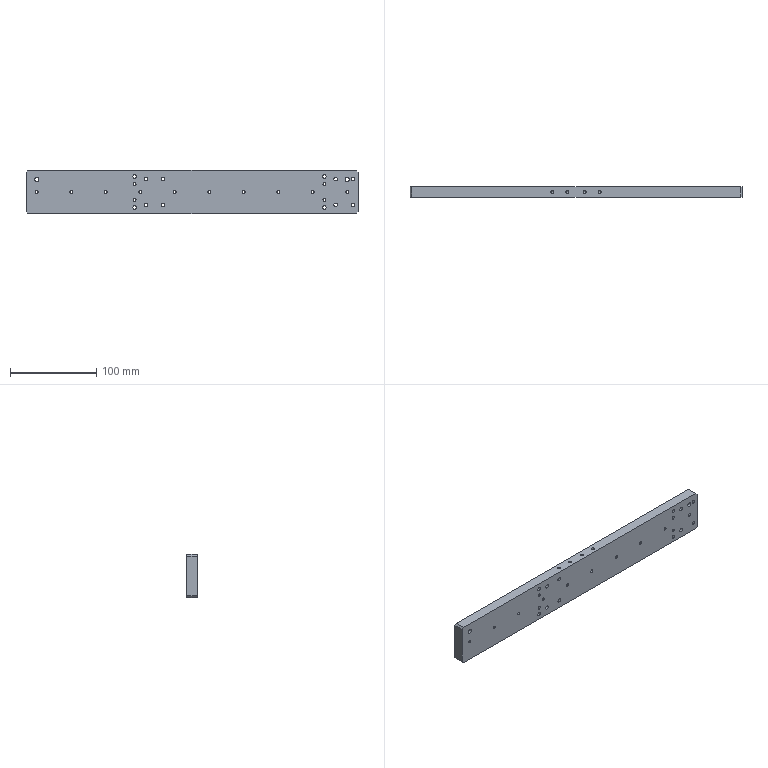Part | 1 solid | 50 faces | box 385 x 12 x 50 mm | volume 226445 mm3 | cylinder 34 | plane 10 | cone 6 | commonest cylinder face diameters 3.3 x20 4.2 x8 4 x4 5 x2
STEP:
#1=CARTESIAN_POINT('',(192.5,-6.,48.));
#2=VERTEX_POINT('',#1);
#3=CARTESIAN_POINT('',(190.5,-6.,50.));
#4=VERTEX_POINT('',#3);
#5=CARTESIAN_POINT('',(190.5,-6.,50.));
#6=DIRECTION('',(-0.7071,0.,0.7071));
#7=VECTOR('',#6,1000.);
#8=LINE('',#5,#7);
#9=EDGE_CURVE('',#2,#4,#8,.T.);
#10=ORIENTED_EDGE('',*,*,#9,.F.);
#11=CARTESIAN_POINT('',(192.5,6.,48.));
#12=VERTEX_POINT('',#11);
#13=CARTESIAN_POINT('',(192.5,-6.,48.));
#14=DIRECTION('',(0.,-1.,0.));
#15=VECTOR('',#14,1000.);
#16=LINE('',#13,#15);
#17=EDGE_CURVE('',#12,#2,#16,.T.);
#18=ORIENTED_EDGE('',*,*,#17,.F.);
#19=CARTESIAN_POINT('',(190.5,6.,50.));
#20=VERTEX_POINT('',#19);
#21=CARTESIAN_POINT('',(190.5,6.,50.));
#22=DIRECTION('',(0.7071,0.,-0.7071));
#23=VECTOR('',#22,1000.);
#24=LINE('',#21,#23);
#25=EDGE_CURVE('',#20,#12,#24,.T.);
#26=ORIENTED_EDGE('',*,*,#25,.F.);
#27=CARTESIAN_POINT('',(190.5,0.,50.));
#28=DIRECTION('',(0.,1.,0.));
#29=VECTOR('',#28,1000.);
#30=LINE('',#27,#29);
#31=EDGE_CURVE('',#4,#20,#30,.T.);
#32=ORIENTED_EDGE('',*,*,#31,.F.);
#33=EDGE_LOOP('',(#10,#18,#26,#32));
#34=FACE_BOUND('',#33,.T.);
#35=CARTESIAN_POINT('',(190.5,0.,50.));
#36=DIRECTION('',(-0.7071,0.,-0.7071));
#37=DIRECTION('',(0.,1.,0.));
#38=AXIS2_PLACEMENT_3D('',#35,#36,#37);
#39=PLANE('',#38);
#40=ADVANCED_FACE('',(#34),#39,.F.);
#41=CARTESIAN_POINT('',(190.5,-6.,0.));
#42=VERTEX_POINT('',#41);
#43=CARTESIAN_POINT('',(192.5,-6.,2.));
#44=VERTEX_POINT('',#43);
#45=CARTESIAN_POINT('',(192.5,-6.,2.));
#46=DIRECTION('',(0.7071,0.,0.7071));
#47=VECTOR('',#46,1000.);
#48=LINE('',#45,#47);
#49=EDGE_CURVE('',#42,#44,#48,.T.);
#50=ORIENTED_EDGE('',*,*,#49,.F.);
#51=CARTESIAN_POINT('',(190.5,6.,0.));
#52=VERTEX_POINT('',#51);
#53=CARTESIAN_POINT('',(190.5,-6.,0.));
#54=DIRECTION('',(0.,-1.,0.));
#55=VECTOR('',#54,1000.);
#56=LINE('',#53,#55);
#57=EDGE_CURVE('',#52,#42,#56,.T.);
#58=ORIENTED_EDGE('',*,*,#57,.F.);
#59=CARTESIAN_POINT('',(192.5,6.,2.));
#60=VERTEX_POINT('',#59);
#61=CARTESIAN_POINT('',(192.5,6.,2.));
#62=DIRECTION('',(-0.7071,0.,-0.7071));
#63=VECTOR('',#62,1000.);
#64=LINE('',#61,#63);
#65=EDGE_CURVE('',#60,#52,#64,.T.);
#66=ORIENTED_EDGE('',*,*,#65,.F.);
#67=CARTESIAN_POINT('',(192.5,6.,2.));
#68=DIRECTION('',(0.,1.,0.));
#69=VECTOR('',#68,1000.);
#70=LINE('',#67,#69);
#71=EDGE_CURVE('',#44,#60,#70,.T.);
#72=ORIENTED_EDGE('',*,*,#71,.F.);
#73=EDGE_LOOP('',(#50,#58,#66,#72));
#74=FACE_BOUND('',#73,.T.);
#75=CARTESIAN_POINT('',(192.5,-6.,2.));
#76=DIRECTION('',(0.7071,0.,-0.7071));
#77=DIRECTION('',(0.,-1.,0.));
#78=AXIS2_PLACEMENT_3D('',#75,#76,#77);
#79=PLANE('',#78);
#80=ADVANCED_FACE('',(#74),#79,.T.);
#81=CARTESIAN_POINT('',(-192.5,6.,48.));
#82=VERTEX_POINT('',#81);
#83=CARTESIAN_POINT('',(-190.5,6.,50.));
#84=VERTEX_POINT('',#83);
#85=CARTESIAN_POINT('',(-190.5,6.,50.));
#86=DIRECTION('',(0.7071,0.,0.7071));
#87=VECTOR('',#86,1000.);
#88=LINE('',#85,#87);
#89=EDGE_CURVE('',#82,#84,#88,.T.);
#90=ORIENTED_EDGE('',*,*,#89,.F.);
#91=CARTESIAN_POINT('',(-192.5,-6.,48.));
#92=VERTEX_POINT('',#91);
#93=CARTESIAN_POINT('',(-192.5,-6.,48.));
#94=DIRECTION('',(0.,1.,0.));
#95=VECTOR('',#94,1000.);
#96=LINE('',#93,#95);
#97=EDGE_CURVE('',#92,#82,#96,.T.);
#98=ORIENTED_EDGE('',*,*,#97,.F.);
#99=CARTESIAN_POINT('',(-190.5,-6.,50.));
#100=VERTEX_POINT('',#99);
#101=CARTESIAN_POINT('',(-190.5,-6.,50.));
#102=DIRECTION('',(-0.7071,0.,-0.7071));
#103=VECTOR('',#102,1000.);
#104=LINE('',#101,#103);
#105=EDGE_CURVE('',#100,#92,#104,.T.);
#106=ORIENTED_EDGE('',*,*,#105,.F.);
#107=CARTESIAN_POINT('',(-190.5,0.,50.));
#108=DIRECTION('',(0.,-1.,0.));
#109=VECTOR('',#108,1000.);
#110=LINE('',#107,#109);
#111=EDGE_CURVE('',#84,#100,#110,.T.);
#112=ORIENTED_EDGE('',*,*,#111,.F.);
#113=EDGE_LOOP('',(#90,#98,#106,#112));
#114=FACE_BOUND('',#113,.T.);
#115=CARTESIAN_POINT('',(-190.5,0.,50.));
#116=DIRECTION('',(0.7071,0.,-0.7071));
#117=DIRECTION('',(0.,-1.,0.));
#118=AXIS2_PLACEMENT_3D('',#115,#116,#117);
#119=PLANE('',#118);
#120=ADVANCED_FACE('',(#114),#119,.F.);
#121=CARTESIAN_POINT('',(-190.5,6.,0.));
#122=VERTEX_POINT('',#121);
#123=CARTESIAN_POINT('',(-192.5,6.,2.));
#124=VERTEX_POINT('',#123);
#125=CARTESIAN_POINT('',(-192.5,6.,2.));
#126=DIRECTION('',(-0.7071,0.,0.7071));
#127=VECTOR('',#126,1000.);
#128=LINE('',#125,#127);
#129=EDGE_CURVE('',#122,#124,#128,.T.);
#130=ORIENTED_EDGE('',*,*,#129,.F.);
#131=CARTESIAN_POINT('',(-190.5,-6.,0.));
#132=VERTEX_POINT('',#131);
#133=CARTESIAN_POINT('',(-190.5,6.,0.));
#134=DIRECTION('',(0.,1.,0.));
#135=VECTOR('',#134,1000.);
#136=LINE('',#133,#135);
#137=EDGE_CURVE('',#132,#122,#136,.T.);
#138=ORIENTED_EDGE('',*,*,#137,.F.);
#139=CARTESIAN_POINT('',(-192.5,-6.,2.));
#140=VERTEX_POINT('',#139);
#141=CARTESIAN_POINT('',(-192.5,-6.,2.));
#142=DIRECTION('',(0.7071,0.,-0.7071));
#143=VECTOR('',#142,1000.);
#144=LINE('',#141,#143);
#145=EDGE_CURVE('',#140,#132,#144,.T.);
#146=ORIENTED_EDGE('',*,*,#145,.F.);
#147=CARTESIAN_POINT('',(-192.5,-6.,2.));
#148=DIRECTION('',(0.,-1.,0.));
#149=VECTOR('',#148,1000.);
#150=LINE('',#147,#149);
#151=EDGE_CURVE('',#124,#140,#150,.T.);
#152=ORIENTED_EDGE('',*,*,#151,.F.);
#153=EDGE_LOOP('',(#130,#138,#146,#152));
#154=FACE_BOUND('',#153,.T.);
#155=CARTESIAN_POINT('',(-192.5,-6.,2.));
#156=DIRECTION('',(-0.7071,0.,-0.7071));
#157=DIRECTION('',(0.,1.,0.));
#158=AXIS2_PLACEMENT_3D('',#155,#156,#157);
#159=PLANE('',#158);
#160=ADVANCED_FACE('',(#154),#159,.T.);
#161=CARTESIAN_POINT('',(-192.5,-6.,0.));
#162=DIRECTION('',(1.,0.,0.));
#163=VECTOR('',#162,1000.);
#164=LINE('',#161,#163);
#165=EDGE_CURVE('',#132,#42,#164,.T.);
#166=ORIENTED_EDGE('',*,*,#165,.F.);
#167=ORIENTED_EDGE('',*,*,#137,.T.);
#168=CARTESIAN_POINT('',(-192.5,6.,0.));
#169=DIRECTION('',(-1.,0.,0.));
#170=VECTOR('',#169,1000.);
#171=LINE('',#168,#170);
#172=EDGE_CURVE('',#52,#122,#171,.T.);
#173=ORIENTED_EDGE('',*,*,#172,.F.);
#174=ORIENTED_EDGE('',*,*,#57,.T.);
#175=EDGE_LOOP('',(#166,#167,#173,#174));
#176=FACE_BOUND('',#175,.T.);
#177=CARTESIAN_POINT('',(-6.65,0.,0.));
#178=VERTEX_POINT('',#177);
#179=CARTESIAN_POINT('',(-5.,0.,0.));
#180=DIRECTION('',(0.,0.,-1.));
#181=DIRECTION('',(-1.,0.,0.));
#182=AXIS2_PLACEMENT_3D('',#179,#180,#181);
#183=CIRCLE('',#182,1.65);
#184=EDGE_CURVE('',#178,#178,#183,.T.);
#185=ORIENTED_EDGE('',*,*,#184,.F.);
#186=EDGE_LOOP('',(#185));
#187=FACE_BOUND('',#186,.T.);
#188=CARTESIAN_POINT('',(3.35,0.,0.));
#189=VERTEX_POINT('',#188);
#190=CARTESIAN_POINT('',(5.,0.,0.));
#191=DIRECTION('',(0.,0.,-1.));
#192=DIRECTION('',(-1.,0.,0.));
#193=AXIS2_PLACEMENT_3D('',#190,#191,#192);
#194=CIRCLE('',#193,1.65);
#195=EDGE_CURVE('',#189,#189,#194,.T.);
#196=ORIENTED_EDGE('',*,*,#195,.F.);
#197=EDGE_LOOP('',(#196));
#198=FACE_BOUND('',#197,.T.);
#199=CARTESIAN_POINT('',(0.,0.,0.));
#200=DIRECTION('',(0.,0.,-1.));
#201=DIRECTION('',(-1.,0.,0.));
#202=AXIS2_PLACEMENT_3D('',#199,#200,#201);
#203=PLANE('',#202);
#204=ADVANCED_FACE('',(#176,#187,#198),#203,.T.);
#205=CARTESIAN_POINT('',(-192.5,-6.,50.));
#206=DIRECTION('',(0.,0.,-1.));
#207=VECTOR('',#206,1000.);
#208=LINE('',#205,#207);
#209=EDGE_CURVE('',#92,#140,#208,.T.);
#210=ORIENTED_EDGE('',*,*,#209,.T.);
#211=ORIENTED_EDGE('',*,*,#145,.T.);
#212=ORIENTED_EDGE('',*,*,#165,.T.);
#213=ORIENTED_EDGE('',*,*,#49,.T.);
#214=CARTESIAN_POINT('',(192.5,-6.,50.));
#215=DIRECTION('',(0.,0.,-1.));
#216=VECTOR('',#215,1000.);
#217=LINE('',#214,#216);
#218=EDGE_CURVE('',#2,#44,#217,.T.);
#219=ORIENTED_EDGE('',*,*,#218,.F.);
#220=ORIENTED_EDGE('',*,*,#9,.T.);
#221=CARTESIAN_POINT('',(-192.5,-6.,50.));
#222=DIRECTION('',(1.,0.,0.));
#223=VECTOR('',#222,1000.);
#224=LINE('',#221,#223);
#225=EDGE_CURVE('',#100,#4,#224,.T.);
#226=ORIENTED_EDGE('',*,*,#225,.F.);
#227=ORIENTED_EDGE('',*,*,#105,.T.);
#228=EDGE_LOOP('',(#210,#211,#212,#213,#219,#220,#226,#227));
#229=FACE_BOUND('',#228,.T.);
#230=CARTESIAN_POINT('',(-180.,-6.,42.));
#231=VERTEX_POINT('',#230);
#232=CARTESIAN_POINT('',(-180.,-6.,39.5));
#233=DIRECTION('',(0.,1.,0.));
#234=DIRECTION('',(0.,0.,1.));
#235=AXIS2_PLACEMENT_3D('',#232,#233,#234);
#236=CIRCLE('',#235,2.5);
#237=EDGE_CURVE('',#231,#231,#236,.T.);
#238=ORIENTED_EDGE('',*,*,#237,.T.);
#239=EDGE_LOOP('',(#238));
#240=FACE_BOUND('',#239,.T.);
#241=CARTESIAN_POINT('',(180.,-6.,42.));
#242=VERTEX_POINT('',#241);
#243=CARTESIAN_POINT('',(180.,-6.,39.5));
#244=DIRECTION('',(0.,1.,0.));
#245=DIRECTION('',(0.,0.,1.));
#246=AXIS2_PLACEMENT_3D('',#243,#244,#245);
#247=CIRCLE('',#246,2.5);
#248=EDGE_CURVE('',#242,#242,#247,.T.);
#249=ORIENTED_EDGE('',*,*,#248,.T.);
#250=EDGE_LOOP('',(#249));
#251=FACE_BOUND('',#250,.T.);
#252=CARTESIAN_POINT('',(180.,-6.,26.65));
#253=VERTEX_POINT('',#252);
#254=CARTESIAN_POINT('',(180.,-6.,25.));
#255=DIRECTION('',(0.,1.,0.));
#256=DIRECTION('',(0.,0.,1.));
#257=AXIS2_PLACEMENT_3D('',#254,#255,#256);
#258=CIRCLE('',#257,1.65);
#259=EDGE_CURVE('',#253,#253,#258,.T.);
#260=ORIENTED_EDGE('',*,*,#259,.T.);
#261=EDGE_LOOP('',(#260));
#262=FACE_BOUND('',#261,.T.);
#263=CARTESIAN_POINT('',(140.,-6.,26.65));
#264=VERTEX_POINT('',#263);
#265=CARTESIAN_POINT('',(140.,-6.,25.));
#266=DIRECTION('',(0.,1.,0.));
#267=DIRECTION('',(0.,0.,1.));
#268=AXIS2_PLACEMENT_3D('',#265,#266,#267);
#269=CIRCLE('',#268,1.65);
#270=EDGE_CURVE('',#264,#264,#269,.T.);
#271=ORIENTED_EDGE('',*,*,#270,.T.);
#272=EDGE_LOOP('',(#271));
#273=FACE_BOUND('',#272,.T.);
#274=CARTESIAN_POINT('',(100.,-6.,26.65));
#275=VERTEX_POINT('',#274);
#276=CARTESIAN_POINT('',(100.,-6.,25.));
#277=DIRECTION('',(0.,1.,0.));
#278=DIRECTION('',(0.,0.,1.));
#279=AXIS2_PLACEMENT_3D('',#276,#277,#278);
#280=CIRCLE('',#279,1.65);
#281=EDGE_CURVE('',#275,#275,#280,.T.);
#282=ORIENTED_EDGE('',*,*,#281,.T.);
#283=EDGE_LOOP('',(#282));
#284=FACE_BOUND('',#283,.T.);
#285=CARTESIAN_POINT('',(60.,-6.,26.65));
#286=VERTEX_POINT('',#285);
#287=CARTESIAN_POINT('',(60.,-6.,25.));
#288=DIRECTION('',(0.,1.,0.));
#289=DIRECTION('',(0.,0.,1.));
#290=AXIS2_PLACEMENT_3D('',#287,#288,#289);
#291=CIRCLE('',#290,1.65);
#292=EDGE_CURVE('',#286,#286,#291,.T.);
#293=ORIENTED_EDGE('',*,*,#292,.T.);
#294=EDGE_LOOP('',(#293));
#295=FACE_BOUND('',#294,.T.);
#296=CARTESIAN_POINT('',(20.,-6.,26.65));
#297=VERTEX_POINT('',#296);
#298=CARTESIAN_POINT('',(20.,-6.,25.));
#299=DIRECTION('',(0.,1.,0.));
#300=DIRECTION('',(0.,0.,1.));
#301=AXIS2_PLACEMENT_3D('',#298,#299,#300);
#302=CIRCLE('',#301,1.65);
#303=EDGE_CURVE('',#297,#297,#302,.T.);
#304=ORIENTED_EDGE('',*,*,#303,.T.);
#305=EDGE_LOOP('',(#304));
#306=FACE_BOUND('',#305,.T.);
#307=CARTESIAN_POINT('',(-20.,-6.,26.65));
#308=VERTEX_POINT('',#307);
#309=CARTESIAN_POINT('',(-20.,-6.,25.));
#310=DIRECTION('',(0.,1.,0.));
#311=DIRECTION('',(0.,0.,1.));
#312=AXIS2_PLACEMENT_3D('',#309,#310,#311);
#313=CIRCLE('',#312,1.65);
#314=EDGE_CURVE('',#308,#308,#313,.T.);
#315=ORIENTED_EDGE('',*,*,#314,.T.);
#316=EDGE_LOOP('',(#315));
#317=FACE_BOUND('',#316,.T.);
#318=CARTESIAN_POINT('',(-60.,-6.,26.65));
#319=VERTEX_POINT('',#318);
#320=CARTESIAN_POINT('',(-60.,-6.,25.));
#321=DIRECTION('',(0.,1.,0.));
#322=DIRECTION('',(0.,0.,1.));
#323=AXIS2_PLACEMENT_3D('',#320,#321,#322);
#324=CIRCLE('',#323,1.65);
#325=EDGE_CURVE('',#319,#319,#324,.T.);
#326=ORIENTED_EDGE('',*,*,#325,.T.);
#327=EDGE_LOOP('',(#326));
#328=FACE_BOUND('',#327,.T.);
#329=CARTESIAN_POINT('',(-100.,-6.,26.65));
#330=VERTEX_POINT('',#329);
#331=CARTESIAN_POINT('',(-100.,-6.,25.));
#332=DIRECTION('',(0.,1.,0.));
#333=DIRECTION('',(0.,0.,1.));
#334=AXIS2_PLACEMENT_3D('',#331,#332,#333);
#335=CIRCLE('',#334,1.65);
#336=EDGE_CURVE('',#330,#330,#335,.T.);
#337=ORIENTED_EDGE('',*,*,#336,.T.);
#338=EDGE_LOOP('',(#337));
#339=FACE_BOUND('',#338,.T.);
#340=CARTESIAN_POINT('',(-140.,-6.,26.65));
#341=VERTEX_POINT('',#340);
#342=CARTESIAN_POINT('',(-140.,-6.,25.));
#343=DIRECTION('',(0.,1.,0.));
#344=DIRECTION('',(0.,0.,1.));
#345=AXIS2_PLACEMENT_3D('',#342,#343,#344);
#346=CIRCLE('',#345,1.65);
#347=EDGE_CURVE('',#341,#341,#346,.T.);
#348=ORIENTED_EDGE('',*,*,#347,.T.);
#349=EDGE_LOOP('',(#348));
#350=FACE_BOUND('',#349,.T.);
#351=CARTESIAN_POINT('',(-180.,-6.,26.65));
#352=VERTEX_POINT('',#351);
#353=CARTESIAN_POINT('',(-180.,-6.,25.));
#354=DIRECTION('',(0.,1.,0.));
#355=DIRECTION('',(0.,0.,1.));
#356=AXIS2_PLACEMENT_3D('',#353,#354,#355);
#357=CIRCLE('',#356,1.65);
#358=EDGE_CURVE('',#352,#352,#357,.T.);
#359=ORIENTED_EDGE('',*,*,#358,.T.);
#360=EDGE_LOOP('',(#359));
#361=FACE_BOUND('',#360,.T.);
#362=CARTESIAN_POINT('',(166.5,-6.,37.9));
#363=VERTEX_POINT('',#362);
#364=CARTESIAN_POINT('',(166.5,-6.,40.));
#365=DIRECTION('',(0.,-1.,0.));
#366=DIRECTION('',(0.,0.,-1.));
#367=AXIS2_PLACEMENT_3D('',#364,#365,#366);
#368=CIRCLE('',#367,2.1);
#369=EDGE_CURVE('',#363,#363,#368,.T.);
#370=ORIENTED_EDGE('',*,*,#369,.F.);
#371=EDGE_LOOP('',(#370));
#372=FACE_BOUND('',#371,.T.);
#373=CARTESIAN_POINT('',(166.5,-6.,7.9));
#374=VERTEX_POINT('',#373);
#375=CARTESIAN_POINT('',(166.5,-6.,10.));
#376=DIRECTION('',(0.,-1.,0.));
#377=DIRECTION('',(0.,0.,-1.));
#378=AXIS2_PLACEMENT_3D('',#375,#376,#377);
#379=CIRCLE('',#378,2.1);
#380=EDGE_CURVE('',#374,#374,#379,.T.);
#381=ORIENTED_EDGE('',*,*,#380,.F.);
#382=EDGE_LOOP('',(#381));
#383=FACE_BOUND('',#382,.T.);
#384=CARTESIAN_POINT('',(186.5,-6.,7.9));
#385=VERTEX_POINT('',#384);
#386=CARTESIAN_POINT('',(186.5,-6.,10.));
#387=DIRECTION('',(0.,-1.,0.));
#388=DIRECTION('',(0.,0.,-1.));
#389=AXIS2_PLACEMENT_3D('',#386,#387,#388);
#390=CIRCLE('',#389,2.1);
#391=EDGE_CURVE('',#385,#385,#390,.T.);
#392=ORIENTED_EDGE('',*,*,#391,.F.);
#393=EDGE_LOOP('',(#392));
#394=FACE_BOUND('',#393,.T.);
#395=CARTESIAN_POINT('',(186.5,-6.,37.9));
#396=VERTEX_POINT('',#395);
#397=CARTESIAN_POINT('',(186.5,-6.,40.));
#398=DIRECTION('',(0.,-1.,0.));
#399=DIRECTION('',(0.,0.,-1.));
#400=AXIS2_PLACEMENT_3D('',#397,#398,#399);
#401=CIRCLE('',#400,2.1);
#402=EDGE_CURVE('',#396,#396,#401,.T.);
#403=ORIENTED_EDGE('',*,*,#402,.F.);
#404=EDGE_LOOP('',(#403));
#405=FACE_BOUND('',#404,.T.);
#406=CARTESIAN_POINT('',(-53.5,-6.,37.9));
#407=VERTEX_POINT('',#406);
#408=CARTESIAN_POINT('',(-53.5,-6.,40.));
#409=DIRECTION('',(0.,-1.,0.));
#410=DIRECTION('',(0.,0.,-1.));
#411=AXIS2_PLACEMENT_3D('',#408,#409,#410);
#412=CIRCLE('',#411,2.1);
#413=EDGE_CURVE('',#407,#407,#412,.T.);
#414=ORIENTED_EDGE('',*,*,#413,.F.);
#415=EDGE_LOOP('',(#414));
#416=FACE_BOUND('',#415,.T.);
#417=CARTESIAN_POINT('',(-53.5,-6.,7.9));
#418=VERTEX_POINT('',#417);
#419=CARTESIAN_POINT('',(-53.5,-6.,10.));
#420=DIRECTION('',(0.,-1.,0.));
#421=DIRECTION('',(0.,0.,-1.));
#422=AXIS2_PLACEMENT_3D('',#419,#420,#421);
#423=CIRCLE('',#422,2.1);
#424=EDGE_CURVE('',#418,#418,#423,.T.);
#425=ORIENTED_EDGE('',*,*,#424,.F.);
#426=EDGE_LOOP('',(#425));
#427=FACE_BOUND('',#426,.T.);
#428=CARTESIAN_POINT('',(-33.5,-6.,7.9));
#429=VERTEX_POINT('',#428);
#430=CARTESIAN_POINT('',(-33.5,-6.,10.));
#431=DIRECTION('',(0.,-1.,0.));
#432=DIRECTION('',(0.,0.,-1.));
#433=AXIS2_PLACEMENT_3D('',#430,#431,#432);
#434=CIRCLE('',#433,2.1);
#435=EDGE_CURVE('',#429,#429,#434,.T.);
#436=ORIENTED_EDGE('',*,*,#435,.F.);
#437=EDGE_LOOP('',(#436));
#438=FACE_BOUND('',#437,.T.);
#439=CARTESIAN_POINT('',(-33.5,-6.,37.9));
#440=VERTEX_POINT('',#439);
#441=CARTESIAN_POINT('',(-33.5,-6.,40.));
#442=DIRECTION('',(0.,-1.,0.));
#443=DIRECTION('',(0.,0.,-1.));
#444=AXIS2_PLACEMENT_3D('',#441,#442,#443);
#445=CIRCLE('',#444,2.1);
#446=EDGE_CURVE('',#440,#440,#445,.T.);
#447=ORIENTED_EDGE('',*,*,#446,.F.);
#448=EDGE_LOOP('',(#447));
#449=FACE_BOUND('',#448,.T.);
#450=CARTESIAN_POINT('',(153.5,-6.,14.35));
#451=VERTEX_POINT('',#450);
#452=CARTESIAN_POINT('',(153.5,-6.,16.));
#453=DIRECTION('',(0.,-1.,0.));
#454=DIRECTION('',(0.,0.,-1.));
#455=AXIS2_PLACEMENT_3D('',#452,#453,#454);
#456=CIRCLE('',#455,1.65);
#457=EDGE_CURVE('',#451,#451,#456,.T.);
#458=ORIENTED_EDGE('',*,*,#457,.F.);
#459=EDGE_LOOP('',(#458));
#460=FACE_BOUND('',#459,.T.);
#461=CARTESIAN_POINT('',(153.5,-6.,32.35));
#462=VERTEX_POINT('',#461);
#463=CARTESIAN_POINT('',(153.5,-6.,34.));
#464=DIRECTION('',(0.,-1.,0.));
#465=DIRECTION('',(0.,0.,-1.));
#466=AXIS2_PLACEMENT_3D('',#463,#464,#465);
#467=CIRCLE('',#466,1.65);
#468=EDGE_CURVE('',#462,#462,#467,.T.);
#469=ORIENTED_EDGE('',*,*,#468,.F.);
#470=EDGE_LOOP('',(#469));
#471=FACE_BOUND('',#470,.T.);
#472=CARTESIAN_POINT('',(-66.5,-6.,14.35));
#473=VERTEX_POINT('',#472);
#474=CARTESIAN_POINT('',(-66.5,-6.,16.));
#475=DIRECTION('',(0.,-1.,0.));
#476=DIRECTION('',(0.,0.,-1.));
#477=AXIS2_PLACEMENT_3D('',#474,#475,#476);
#478=CIRCLE('',#477,1.65);
#479=EDGE_CURVE('',#473,#473,#478,.T.);
#480=ORIENTED_EDGE('',*,*,#479,.F.);
#481=EDGE_LOOP('',(#480));
#482=FACE_BOUND('',#481,.T.);
#483=CARTESIAN_POINT('',(-66.5,-6.,32.35));
#484=VERTEX_POINT('',#483);
#485=CARTESIAN_POINT('',(-66.5,-6.,34.));
#486=DIRECTION('',(0.,-1.,0.));
#487=DIRECTION('',(0.,0.,-1.));
#488=AXIS2_PLACEMENT_3D('',#485,#486,#487);
#489=CIRCLE('',#488,1.65);
#490=EDGE_CURVE('',#484,#484,#489,.T.);
#491=ORIENTED_EDGE('',*,*,#490,.F.);
#492=EDGE_LOOP('',(#491));
#493=FACE_BOUND('',#492,.T.);
#494=CARTESIAN_POINT('',(153.5,-6.,5.));
#495=VERTEX_POINT('',#494);
#496=CARTESIAN_POINT('',(153.5,-6.,7.));
#497=DIRECTION('',(0.,-1.,0.));
#498=DIRECTION('',(0.,0.,-1.));
#499=AXIS2_PLACEMENT_3D('',#496,#497,#498);
#500=CIRCLE('',#499,2.);
#501=EDGE_CURVE('',#495,#495,#500,.T.);
#502=ORIENTED_EDGE('',*,*,#501,.F.);
#503=EDGE_LOOP('',(#502));
#504=FACE_BOUND('',#503,.T.);
#505=CARTESIAN_POINT('',(153.5,-6.,41.));
#506=VERTEX_POINT('',#505);
#507=CARTESIAN_POINT('',(153.5,-6.,43.));
#508=DIRECTION('',(0.,-1.,0.));
#509=DIRECTION('',(0.,0.,-1.));
#510=AXIS2_PLACEMENT_3D('',#507,#508,#509);
#511=CIRCLE('',#510,2.);
#512=EDGE_CURVE('',#506,#506,#511,.T.);
#513=ORIENTED_EDGE('',*,*,#512,.F.);
#514=EDGE_LOOP('',(#513));
#515=FACE_BOUND('',#514,.T.);
#516=CARTESIAN_POINT('',(-66.5,-6.,41.));
#517=VERTEX_POINT('',#516);
#518=CARTESIAN_POINT('',(-66.5,-6.,43.));
#519=DIRECTION('',(0.,-1.,0.));
#520=DIRECTION('',(0.,0.,-1.));
#521=AXIS2_PLACEMENT_3D('',#518,#519,#520);
#522=CIRCLE('',#521,2.);
#523=EDGE_CURVE('',#517,#517,#522,.T.);
#524=ORIENTED_EDGE('',*,*,#523,.F.);
#525=EDGE_LOOP('',(#524));
#526=FACE_BOUND('',#525,.T.);
#527=CARTESIAN_POINT('',(-66.5,-6.,5.));
#528=VERTEX_POINT('',#527);
#529=CARTESIAN_POINT('',(-66.5,-6.,7.));
#530=DIRECTION('',(0.,-1.,0.));
#531=DIRECTION('',(0.,0.,-1.));
#532=AXIS2_PLACEMENT_3D('',#529,#530,#531);
#533=CIRCLE('',#532,2.);
#534=EDGE_CURVE('',#528,#528,#533,.T.);
#535=ORIENTED_EDGE('',*,*,#534,.F.);
#536=EDGE_LOOP('',(#535));
#537=FACE_BOUND('',#536,.T.);
#538=CARTESIAN_POINT('',(-192.5,-6.,50.));
#539=DIRECTION('',(0.,1.,0.));
#540=DIRECTION('',(0.,0.,1.));
#541=AXIS2_PLACEMENT_3D('',#538,#539,#540);
#542=PLANE('',#541);
#543=ADVANCED_FACE('',(#229,#240,#251,#262,#273,#284,#295,#306,#317,#328,#339,#350,#361,#372,#383,#394,#405,#416,#427,#438,#449,#460,#471,#482,#493,#504,#515,#526,#537),#542,.F.);
#544=CARTESIAN_POINT('',(-192.5,6.,50.));
#545=DIRECTION('',(0.,0.,-1.));
#546=VECTOR('',#545,1000.);
#547=LINE('',#544,#546);
#548=EDGE_CURVE('',#82,#124,#547,.T.);
#549=ORIENTED_EDGE('',*,*,#548,.T.);
#550=ORIENTED_EDGE('',*,*,#151,.T.);
#551=ORIENTED_EDGE('',*,*,#209,.F.);
#552=ORIENTED_EDGE('',*,*,#97,.T.);
#553=EDGE_LOOP('',(#549,#550,#551,#552));
#554=FACE_BOUND('',#553,.T.);
#555=CARTESIAN_POINT('',(-192.5,-6.,50.));
#556=DIRECTION('',(1.,0.,0.));
#557=DIRECTION('',(0.,0.,-1.));
#558=AXIS2_PLACEMENT_3D('',#555,#556,#557);
#559=PLANE('',#558);
#560=ADVANCED_FACE('',(#554),#559,.F.);
#561=ORIENTED_EDGE('',*,*,#172,.T.);
#562=ORIENTED_EDGE('',*,*,#129,.T.);
#563=ORIENTED_EDGE('',*,*,#548,.F.);
#564=ORIENTED_EDGE('',*,*,#89,.T.);
#565=CARTESIAN_POINT('',(-192.5,6.,50.));
#566=DIRECTION('',(-1.,0.,0.));
#567=VECTOR('',#566,1000.);
#568=LINE('',#565,#567);
#569=EDGE_CURVE('',#20,#84,#568,.T.);
#570=ORIENTED_EDGE('',*,*,#569,.F.);
#571=ORIENTED_EDGE('',*,*,#25,.T.);
#572=CARTESIAN_POINT('',(192.5,6.,50.));
#573=DIRECTION('',(0.,0.,-1.));
#574=VECTOR('',#573,1000.);
#575=LINE('',#572,#574);
#576=EDGE_CURVE('',#12,#60,#575,.T.);
#577=ORIENTED_EDGE('',*,*,#576,.T.);
#578=ORIENTED_EDGE('',*,*,#65,.T.);
#579=EDGE_LOOP('',(#561,#562,#563,#564,#570,#571,#577,#578));
#580=FACE_BOUND('',#579,.T.);
#581=CARTESIAN_POINT('',(-180.,6.,42.));
#582=VERTEX_POINT('',#581);
#583=CARTESIAN_POINT('',(-180.,6.,39.5));
#584=DIRECTION('',(0.,1.,0.));
#585=DIRECTION('',(0.,0.,1.));
#586=AXIS2_PLACEMENT_3D('',#583,#584,#585);
#587=CIRCLE('',#586,2.5);
#588=EDGE_CURVE('',#582,#582,#587,.T.);
#589=ORIENTED_EDGE('',*,*,#588,.F.);
#590=EDGE_LOOP('',(#589));
#591=FACE_BOUND('',#590,.T.);
#592=CARTESIAN_POINT('',(180.,6.,42.));
#593=VERTEX_POINT('',#592);
#594=CARTESIAN_POINT('',(180.,6.,39.5));
#595=DIRECTION('',(0.,1.,0.));
#596=DIRECTION('',(0.,0.,1.));
#597=AXIS2_PLACEMENT_3D('',#594,#595,#596);
#598=CIRCLE('',#597,2.5);
#599=EDGE_CURVE('',#593,#593,#598,.T.);
#600=ORIENTED_EDGE('',*,*,#599,.F.);
#601=EDGE_LOOP('',(#600));
#602=FACE_BOUND('',#601,.T.);
#603=CARTESIAN_POINT('',(180.,6.,26.65));
#604=VERTEX_POINT('',#603);
#605=CARTESIAN_POINT('',(180.,6.,25.));
#606=DIRECTION('',(0.,1.,0.));
#607=DIRECTION('',(0.,0.,1.));
#608=AXIS2_PLACEMENT_3D('',#605,#606,#607);
#609=CIRCLE('',#608,1.65);
#610=EDGE_CURVE('',#604,#604,#609,.T.);
#611=ORIENTED_EDGE('',*,*,#610,.F.);
#612=EDGE_LOOP('',(#611));
#613=FACE_BOUND('',#612,.T.);
#614=CARTESIAN_POINT('',(140.,6.,26.65));
#615=VERTEX_POINT('',#614);
#616=CARTESIAN_POINT('',(140.,6.,25.));
#617=DIRECTION('',(0.,1.,0.));
#618=DIRECTION('',(0.,0.,1.));
#619=AXIS2_PLACEMENT_3D('',#616,#617,#618);
#620=CIRCLE('',#619,1.65);
#621=EDGE_CURVE('',#615,#615,#620,.T.);
#622=ORIENTED_EDGE('',*,*,#621,.F.);
#623=EDGE_LOOP('',(#622));
#624=FACE_BOUND('',#623,.T.);
#625=CARTESIAN_POINT('',(100.,6.,26.65));
#626=VERTEX_POINT('',#625);
#627=CARTESIAN_POINT('',(100.,6.,25.));
#628=DIRECTION('',(0.,1.,0.));
#629=DIRECTION('',(0.,0.,1.));
#630=AXIS2_PLACEMENT_3D('',#627,#628,#629);
#631=CIRCLE('',#630,1.65);
#632=EDGE_CURVE('',#626,#626,#631,.T.);
#633=ORIENTED_EDGE('',*,*,#632,.F.);
#634=EDGE_LOOP('',(#633));
#635=FACE_BOUND('',#634,.T.);
#636=CARTESIAN_POINT('',(60.,6.,26.65));
#637=VERTEX_POINT('',#636);
#638=CARTESIAN_POINT('',(60.,6.,25.));
#639=DIRECTION('',(0.,1.,0.));
#640=DIRECTION('',(0.,0.,1.));
#641=AXIS2_PLACEMENT_3D('',#638,#639,#640);
#642=CIRCLE('',#641,1.65);
#643=EDGE_CURVE('',#637,#637,#642,.T.);
#644=ORIENTED_EDGE('',*,*,#643,.F.);
#645=EDGE_LOOP('',(#644));
#646=FACE_BOUND('',#645,.T.);
#647=CARTESIAN_POINT('',(20.,6.,26.65));
#648=VERTEX_POINT('',#647);
#649=CARTESIAN_POINT('',(20.,6.,25.));
#650=DIRECTION('',(0.,1.,0.));
#651=DIRECTION('',(0.,0.,1.));
#652=AXIS2_PLACEMENT_3D('',#649,#650,#651);
#653=CIRCLE('',#652,1.65);
#654=EDGE_CURVE('',#648,#648,#653,.T.);
#655=ORIENTED_EDGE('',*,*,#654,.F.);
#656=EDGE_LOOP('',(#655));
#657=FACE_BOUND('',#656,.T.);
#658=CARTESIAN_POINT('',(-20.,6.,26.65));
#659=VERTEX_POINT('',#658);
#660=CARTESIAN_POINT('',(-20.,6.,25.));
#661=DIRECTION('',(0.,1.,0.));
#662=DIRECTION('',(0.,0.,1.));
#663=AXIS2_PLACEMENT_3D('',#660,#661,#662);
#664=CIRCLE('',#663,1.65);
#665=EDGE_CURVE('',#659,#659,#664,.T.);
#666=ORIENTED_EDGE('',*,*,#665,.F.);
#667=EDGE_LOOP('',(#666));
#668=FACE_BOUND('',#667,.T.);
#669=CARTESIAN_POINT('',(-60.,6.,26.65));
#670=VERTEX_POINT('',#669);
#671=CARTESIAN_POINT('',(-60.,6.,25.));
#672=DIRECTION('',(0.,1.,0.));
#673=DIRECTION('',(0.,0.,1.));
#674=AXIS2_PLACEMENT_3D('',#671,#672,#673);
#675=CIRCLE('',#674,1.65);
#676=EDGE_CURVE('',#670,#670,#675,.T.);
#677=ORIENTED_EDGE('',*,*,#676,.F.);
#678=EDGE_LOOP('',(#677));
#679=FACE_BOUND('',#678,.T.);
#680=CARTESIAN_POINT('',(-100.,6.,26.65));
#681=VERTEX_POINT('',#680);
#682=CARTESIAN_POINT('',(-100.,6.,25.));
#683=DIRECTION('',(0.,1.,0.));
#684=DIRECTION('',(0.,0.,1.));
#685=AXIS2_PLACEMENT_3D('',#682,#683,#684);
#686=CIRCLE('',#685,1.65);
#687=EDGE_CURVE('',#681,#681,#686,.T.);
#688=ORIENTED_EDGE('',*,*,#687,.F.);
#689=EDGE_LOOP('',(#688));
#690=FACE_BOUND('',#689,.T.);
#691=CARTESIAN_POINT('',(-140.,6.,26.65));
#692=VERTEX_POINT('',#691);
#693=CARTESIAN_POINT('',(-140.,6.,25.));
#694=DIRECTION('',(0.,1.,0.));
#695=DIRECTION('',(0.,0.,1.));
#696=AXIS2_PLACEMENT_3D('',#693,#694,#695);
#697=CIRCLE('',#696,1.65);
#698=EDGE_CURVE('',#692,#692,#697,.T.);
#699=ORIENTED_EDGE('',*,*,#698,.F.);
#700=EDGE_LOOP('',(#699));
#701=FACE_BOUND('',#700,.T.);
#702=CARTESIAN_POINT('',(-180.,6.,26.65));
#703=VERTEX_POINT('',#702);
#704=CARTESIAN_POINT('',(-180.,6.,25.));
#705=DIRECTION('',(0.,1.,0.));
#706=DIRECTION('',(0.,0.,1.));
#707=AXIS2_PLACEMENT_3D('',#704,#705,#706);
#708=CIRCLE('',#707,1.65);
#709=EDGE_CURVE('',#703,#703,#708,.T.);
#710=ORIENTED_EDGE('',*,*,#709,.F.);
#711=EDGE_LOOP('',(#710));
#712=FACE_BOUND('',#711,.T.);
#713=CARTESIAN_POINT('',(166.5,6.,37.9));
#714=VERTEX_POINT('',#713);
#715=CARTESIAN_POINT('',(166.5,6.,40.));
#716=DIRECTION('',(0.,-1.,0.));
#717=DIRECTION('',(0.,0.,-1.));
#718=AXIS2_PLACEMENT_3D('',#715,#716,#717);
#719=CIRCLE('',#718,2.1);
#720=EDGE_CURVE('',#714,#714,#719,.T.);
#721=ORIENTED_EDGE('',*,*,#720,.T.);
#722=EDGE_LOOP('',(#721));
#723=FACE_BOUND('',#722,.T.);
#724=CARTESIAN_POINT('',(166.5,6.,7.9));
#725=VERTEX_POINT('',#724);
#726=CARTESIAN_POINT('',(166.5,6.,10.));
#727=DIRECTION('',(0.,-1.,0.));
#728=DIRECTION('',(0.,0.,-1.));
#729=AXIS2_PLACEMENT_3D('',#726,#727,#728);
#730=CIRCLE('',#729,2.1);
#731=EDGE_CURVE('',#725,#725,#730,.T.);
#732=ORIENTED_EDGE('',*,*,#731,.T.);
#733=EDGE_LOOP('',(#732));
#734=FACE_BOUND('',#733,.T.);
#735=CARTESIAN_POINT('',(186.5,6.,7.9));
#736=VERTEX_POINT('',#735);
#737=CARTESIAN_POINT('',(186.5,6.,10.));
#738=DIRECTION('',(0.,-1.,0.));
#739=DIRECTION('',(0.,0.,-1.));
#740=AXIS2_PLACEMENT_3D('',#737,#738,#739);
#741=CIRCLE('',#740,2.1);
#742=EDGE_CURVE('',#736,#736,#741,.T.);
#743=ORIENTED_EDGE('',*,*,#742,.T.);
#744=EDGE_LOOP('',(#743));
#745=FACE_BOUND('',#744,.T.);
#746=CARTESIAN_POINT('',(186.5,6.,37.9));
#747=VERTEX_POINT('',#746);
#748=CARTESIAN_POINT('',(186.5,6.,40.));
#749=DIRECTION('',(0.,-1.,0.));
#750=DIRECTION('',(0.,0.,-1.));
#751=AXIS2_PLACEMENT_3D('',#748,#749,#750);
#752=CIRCLE('',#751,2.1);
#753=EDGE_CURVE('',#747,#747,#752,.T.);
#754=ORIENTED_EDGE('',*,*,#753,.T.);
#755=EDGE_LOOP('',(#754));
#756=FACE_BOUND('',#755,.T.);
#757=CARTESIAN_POINT('',(-53.5,6.,37.9));
#758=VERTEX_POINT('',#757);
#759=CARTESIAN_POINT('',(-53.5,6.,40.));
#760=DIRECTION('',(0.,-1.,0.));
#761=DIRECTION('',(0.,0.,-1.));
#762=AXIS2_PLACEMENT_3D('',#759,#760,#761);
#763=CIRCLE('',#762,2.1);
#764=EDGE_CURVE('',#758,#758,#763,.T.);
#765=ORIENTED_EDGE('',*,*,#764,.T.);
#766=EDGE_LOOP('',(#765));
#767=FACE_BOUND('',#766,.T.);
#768=CARTESIAN_POINT('',(-53.5,6.,7.9));
#769=VERTEX_POINT('',#768);
#770=CARTESIAN_POINT('',(-53.5,6.,10.));
#771=DIRECTION('',(0.,-1.,0.));
#772=DIRECTION('',(0.,0.,-1.));
#773=AXIS2_PLACEMENT_3D('',#770,#771,#772);
#774=CIRCLE('',#773,2.1);
#775=EDGE_CURVE('',#769,#769,#774,.T.);
#776=ORIENTED_EDGE('',*,*,#775,.T.);
#777=EDGE_LOOP('',(#776));
#778=FACE_BOUND('',#777,.T.);
#779=CARTESIAN_POINT('',(-33.5,6.,7.9));
#780=VERTEX_POINT('',#779);
#781=CARTESIAN_POINT('',(-33.5,6.,10.));
#782=DIRECTION('',(0.,-1.,0.));
#783=DIRECTION('',(0.,0.,-1.));
#784=AXIS2_PLACEMENT_3D('',#781,#782,#783);
#785=CIRCLE('',#784,2.1);
#786=EDGE_CURVE('',#780,#780,#785,.T.);
#787=ORIENTED_EDGE('',*,*,#786,.T.);
#788=EDGE_LOOP('',(#787));
#789=FACE_BOUND('',#788,.T.);
#790=CARTESIAN_POINT('',(-33.5,6.,37.9));
#791=VERTEX_POINT('',#790);
#792=CARTESIAN_POINT('',(-33.5,6.,40.));
#793=DIRECTION('',(0.,-1.,0.));
#794=DIRECTION('',(0.,0.,-1.));
#795=AXIS2_PLACEMENT_3D('',#792,#793,#794);
#796=CIRCLE('',#795,2.1);
#797=EDGE_CURVE('',#791,#791,#796,.T.);
#798=ORIENTED_EDGE('',*,*,#797,.T.);
#799=EDGE_LOOP('',(#798));
#800=FACE_BOUND('',#799,.T.);
#801=CARTESIAN_POINT('',(153.5,6.,14.35));
#802=VERTEX_POINT('',#801);
#803=CARTESIAN_POINT('',(153.5,6.,16.));
#804=DIRECTION('',(0.,-1.,0.));
#805=DIRECTION('',(0.,0.,-1.));
#806=AXIS2_PLACEMENT_3D('',#803,#804,#805);
#807=CIRCLE('',#806,1.65);
#808=EDGE_CURVE('',#802,#802,#807,.T.);
#809=ORIENTED_EDGE('',*,*,#808,.T.);
#810=EDGE_LOOP('',(#809));
#811=FACE_BOUND('',#810,.T.);
#812=CARTESIAN_POINT('',(153.5,6.,32.35));
#813=VERTEX_POINT('',#812);
#814=CARTESIAN_POINT('',(153.5,6.,34.));
#815=DIRECTION('',(0.,-1.,0.));
#816=DIRECTION('',(0.,0.,-1.));
#817=AXIS2_PLACEMENT_3D('',#814,#815,#816);
#818=CIRCLE('',#817,1.65);
#819=EDGE_CURVE('',#813,#813,#818,.T.);
#820=ORIENTED_EDGE('',*,*,#819,.T.);
#821=EDGE_LOOP('',(#820));
#822=FACE_BOUND('',#821,.T.);
#823=CARTESIAN_POINT('',(-66.5,6.,14.35));
#824=VERTEX_POINT('',#823);
#825=CARTESIAN_POINT('',(-66.5,6.,16.));
#826=DIRECTION('',(0.,-1.,0.));
#827=DIRECTION('',(0.,0.,-1.));
#828=AXIS2_PLACEMENT_3D('',#825,#826,#827);
#829=CIRCLE('',#828,1.65);
#830=EDGE_CURVE('',#824,#824,#829,.T.);
#831=ORIENTED_EDGE('',*,*,#830,.T.);
#832=EDGE_LOOP('',(#831));
#833=FACE_BOUND('',#832,.T.);
#834=CARTESIAN_POINT('',(-66.5,6.,32.35));
#835=VERTEX_POINT('',#834);
#836=CARTESIAN_POINT('',(-66.5,6.,34.));
#837=DIRECTION('',(0.,-1.,0.));
#838=DIRECTION('',(0.,0.,-1.));
#839=AXIS2_PLACEMENT_3D('',#836,#837,#838);
#840=CIRCLE('',#839,1.65);
#841=EDGE_CURVE('',#835,#835,#840,.T.);
#842=ORIENTED_EDGE('',*,*,#841,.T.);
#843=EDGE_LOOP('',(#842));
#844=FACE_BOUND('',#843,.T.);
#845=CARTESIAN_POINT('',(153.5,6.,5.));
#846=VERTEX_POINT('',#845);
#847=CARTESIAN_POINT('',(153.5,6.,7.));
#848=DIRECTION('',(0.,-1.,0.));
#849=DIRECTION('',(0.,0.,-1.));
#850=AXIS2_PLACEMENT_3D('',#847,#848,#849);
#851=CIRCLE('',#850,2.);
#852=EDGE_CURVE('',#846,#846,#851,.T.);
#853=ORIENTED_EDGE('',*,*,#852,.T.);
#854=EDGE_LOOP('',(#853));
#855=FACE_BOUND('',#854,.T.);
#856=CARTESIAN_POINT('',(153.5,6.,41.));
#857=VERTEX_POINT('',#856);
#858=CARTESIAN_POINT('',(153.5,6.,43.));
#859=DIRECTION('',(0.,-1.,0.));
#860=DIRECTION('',(0.,0.,-1.));
#861=AXIS2_PLACEMENT_3D('',#858,#859,#860);
#862=CIRCLE('',#861,2.);
#863=EDGE_CURVE('',#857,#857,#862,.T.);
#864=ORIENTED_EDGE('',*,*,#863,.T.);
#865=EDGE_LOOP('',(#864));
#866=FACE_BOUND('',#865,.T.);
#867=CARTESIAN_POINT('',(-66.5,6.,41.));
#868=VERTEX_POINT('',#867);
#869=CARTESIAN_POINT('',(-66.5,6.,43.));
#870=DIRECTION('',(0.,-1.,0.));
#871=DIRECTION('',(0.,0.,-1.));
#872=AXIS2_PLACEMENT_3D('',#869,#870,#871);
#873=CIRCLE('',#872,2.);
#874=EDGE_CURVE('',#868,#868,#873,.T.);
#875=ORIENTED_EDGE('',*,*,#874,.T.);
#876=EDGE_LOOP('',(#875));
#877=FACE_BOUND('',#876,.T.);
#878=CARTESIAN_POINT('',(-66.5,6.,5.));
#879=VERTEX_POINT('',#878);
#880=CARTESIAN_POINT('',(-66.5,6.,7.));
#881=DIRECTION('',(0.,-1.,0.));
#882=DIRECTION('',(0.,0.,-1.));
#883=AXIS2_PLACEMENT_3D('',#880,#881,#882);
#884=CIRCLE('',#883,2.);
#885=EDGE_CURVE('',#879,#879,#884,.T.);
#886=ORIENTED_EDGE('',*,*,#885,.T.);
#887=EDGE_LOOP('',(#886));
#888=FACE_BOUND('',#887,.T.);
#889=CARTESIAN_POINT('',(-192.5,6.,50.));
#890=DIRECTION('',(0.,-1.,0.));
#891=DIRECTION('',(0.,0.,-1.));
#892=AXIS2_PLACEMENT_3D('',#889,#890,#891);
#893=PLANE('',#892);
#894=ADVANCED_FACE('',(#580,#591,#602,#613,#624,#635,#646,#657,#668,#679,#690,#701,#712,#723,#734,#745,#756,#767,#778,#789,#800,#811,#822,#833,#844,#855,#866,#877,#888),#893,.F.);
#895=ORIENTED_EDGE('',*,*,#218,.T.);
#896=ORIENTED_EDGE('',*,*,#71,.T.);
#897=ORIENTED_EDGE('',*,*,#576,.F.);
#898=ORIENTED_EDGE('',*,*,#17,.T.);
#899=EDGE_LOOP('',(#895,#896,#897,#898));
#900=FACE_BOUND('',#899,.T.);
#901=CARTESIAN_POINT('',(192.5,-6.,50.));
#902=DIRECTION('',(-1.,0.,0.));
#903=DIRECTION('',(0.,0.,1.));
#904=AXIS2_PLACEMENT_3D('',#901,#902,#903);
#905=PLANE('',#904);
#906=ADVANCED_FACE('',(#900),#905,.F.);
#907=ORIENTED_EDGE('',*,*,#225,.T.);
#908=ORIENTED_EDGE('',*,*,#31,.T.);
#909=ORIENTED_EDGE('',*,*,#569,.T.);
#910=ORIENTED_EDGE('',*,*,#111,.T.);
#911=EDGE_LOOP('',(#907,#908,#909,#910));
#912=FACE_BOUND('',#911,.T.);
#913=CARTESIAN_POINT('',(29.15,0.,50.));
#914=VERTEX_POINT('',#913);
#915=CARTESIAN_POINT('',(27.5,0.,50.));
#916=DIRECTION('',(0.,0.,1.));
#917=DIRECTION('',(1.,0.,0.));
#918=AXIS2_PLACEMENT_3D('',#915,#916,#917);
#919=CIRCLE('',#918,1.65);
#920=EDGE_CURVE('',#914,#914,#919,.T.);
#921=ORIENTED_EDGE('',*,*,#920,.F.);
#922=EDGE_LOOP('',(#921));
#923=FACE_BOUND('',#922,.T.);
#924=CARTESIAN_POINT('',(8.35,0.,50.));
#925=VERTEX_POINT('',#924);
#926=CARTESIAN_POINT('',(10.,0.,50.));
#927=DIRECTION('',(0.,0.,-1.));
#928=DIRECTION('',(-1.,0.,0.));
#929=AXIS2_PLACEMENT_3D('',#926,#927,#928);
#930=CIRCLE('',#929,1.65);
#931=EDGE_CURVE('',#925,#925,#930,.F.);
#932=ORIENTED_EDGE('',*,*,#931,.F.);
#933=EDGE_LOOP('',(#932));
#934=FACE_BOUND('',#933,.T.);
#935=CARTESIAN_POINT('',(-11.65,0.,50.));
#936=VERTEX_POINT('',#935);
#937=CARTESIAN_POINT('',(-10.,0.,50.));
#938=DIRECTION('',(0.,0.,-1.));
#939=DIRECTION('',(-1.,0.,0.));
#940=AXIS2_PLACEMENT_3D('',#937,#938,#939);
#941=CIRCLE('',#940,1.65);
#942=EDGE_CURVE('',#936,#936,#941,.F.);
#943=ORIENTED_EDGE('',*,*,#942,.F.);
#944=EDGE_LOOP('',(#943));
#945=FACE_BOUND('',#944,.T.);
#946=CARTESIAN_POINT('',(-25.85,0.,50.));
#947=VERTEX_POINT('',#946);
#948=CARTESIAN_POINT('',(-27.5,0.,50.));
#949=DIRECTION('',(0.,0.,1.));
#950=DIRECTION('',(1.,0.,0.));
#951=AXIS2_PLACEMENT_3D('',#948,#949,#950);
#952=CIRCLE('',#951,1.65);
#953=EDGE_CURVE('',#947,#947,#952,.T.);
#954=ORIENTED_EDGE('',*,*,#953,.F.);
#955=EDGE_LOOP('',(#954));
#956=FACE_BOUND('',#955,.T.);
#957=CARTESIAN_POINT('',(0.,0.,50.));
#958=DIRECTION('',(0.,0.,-1.));
#959=DIRECTION('',(-1.,0.,0.));
#960=AXIS2_PLACEMENT_3D('',#957,#958,#959);
#961=PLANE('',#960);
#962=ADVANCED_FACE('',(#912,#923,#934,#945,#956),#961,.F.);
#963=CARTESIAN_POINT('',(11.65,0.,37.9));
#964=VERTEX_POINT('',#963);
#965=CARTESIAN_POINT('',(10.,0.,37.9));
#966=DIRECTION('',(0.,0.,1.));
#967=DIRECTION('',(1.,0.,0.));
#968=AXIS2_PLACEMENT_3D('',#965,#966,#967);
#969=CIRCLE('',#968,1.65);
#970=EDGE_CURVE('',#964,#964,#969,.T.);
#971=ORIENTED_EDGE('',*,*,#970,.T.);
#972=EDGE_LOOP('',(#971));
#973=FACE_BOUND('',#972,.T.);
#974=CARTESIAN_POINT('',(10.,0.,36.909));
#975=VERTEX_POINT('',#974);
#976=VERTEX_LOOP('',#975);
#977=FACE_BOUND('',#976,.T.);
#978=CARTESIAN_POINT('',(10.,0.,37.9));
#979=DIRECTION('',(0.,0.,1.));
#980=DIRECTION('',(1.,0.,0.));
#981=AXIS2_PLACEMENT_3D('',#978,#979,#980);
#982=CONICAL_SURFACE('',#981,1.65,1.03);
#983=ADVANCED_FACE('',(#973,#977),#982,.F.);
#984=ORIENTED_EDGE('',*,*,#970,.F.);
#985=EDGE_LOOP('',(#984));
#986=FACE_BOUND('',#985,.T.);
#987=ORIENTED_EDGE('',*,*,#931,.T.);
#988=EDGE_LOOP('',(#987));
#989=FACE_BOUND('',#988,.T.);
#990=CARTESIAN_POINT('',(10.,0.,48.));
#991=DIRECTION('',(0.,0.,1.));
#992=DIRECTION('',(1.,0.,0.));
#993=AXIS2_PLACEMENT_3D('',#990,#991,#992);
#994=CYLINDRICAL_SURFACE('',#993,1.65);
#995=ADVANCED_FACE('',(#986,#989),#994,.F.);
#996=CARTESIAN_POINT('',(-8.35,0.,37.9));
#997=VERTEX_POINT('',#996);
#998=CARTESIAN_POINT('',(-10.,0.,37.9));
#999=DIRECTION('',(0.,0.,1.));
#1000=DIRECTION('',(1.,0.,0.));
#1001=AXIS2_PLACEMENT_3D('',#998,#999,#1000);
#1002=CIRCLE('',#1001,1.65);
#1003=EDGE_CURVE('',#997,#997,#1002,.T.);
#1004=ORIENTED_EDGE('',*,*,#1003,.T.);
#1005=EDGE_LOOP('',(#1004));
#1006=FACE_BOUND('',#1005,.T.);
#1007=CARTESIAN_POINT('',(-10.,0.,36.909));
#1008=VERTEX_POINT('',#1007);
#1009=VERTEX_LOOP('',#1008);
#1010=FACE_BOUND('',#1009,.T.);
#1011=CARTESIAN_POINT('',(-10.,0.,37.9));
#1012=DIRECTION('',(0.,0.,1.));
#1013=DIRECTION('',(1.,0.,0.));
#1014=AXIS2_PLACEMENT_3D('',#1011,#1012,#1013);
#1015=CONICAL_SURFACE('',#1014,1.65,1.03);
#1016=ADVANCED_FACE('',(#1006,#1010),#1015,.F.);
#1017=ORIENTED_EDGE('',*,*,#1003,.F.);
#1018=EDGE_LOOP('',(#1017));
#1019=FACE_BOUND('',#1018,.T.);
#1020=ORIENTED_EDGE('',*,*,#942,.T.);
#1021=EDGE_LOOP('',(#1020));
#1022=FACE_BOUND('',#1021,.T.);
#1023=CARTESIAN_POINT('',(-10.,0.,48.));
#1024=DIRECTION('',(0.,0.,1.));
#1025=DIRECTION('',(1.,0.,0.));
#1026=AXIS2_PLACEMENT_3D('',#1023,#1024,#1025);
#1027=CYLINDRICAL_SURFACE('',#1026,1.65);
#1028=ADVANCED_FACE('',(#1019,#1022),#1027,.F.);
#1029=ORIENTED_EDGE('',*,*,#237,.F.);
#1030=EDGE_LOOP('',(#1029));
#1031=FACE_BOUND('',#1030,.T.);
#1032=ORIENTED_EDGE('',*,*,#588,.T.);
#1033=EDGE_LOOP('',(#1032));
#1034=FACE_BOUND('',#1033,.T.);
#1035=CARTESIAN_POINT('',(-180.,6.,39.5));
#1036=DIRECTION('',(0.,1.,0.));
#1037=DIRECTION('',(0.,0.,1.));
#1038=AXIS2_PLACEMENT_3D('',#1035,#1036,#1037);
#1039=CYLINDRICAL_SURFACE('',#1038,2.5);
#1040=ADVANCED_FACE('',(#1031,#1034),#1039,.F.);
#1041=ORIENTED_EDGE('',*,*,#248,.F.);
#1042=EDGE_LOOP('',(#1041));
#1043=FACE_BOUND('',#1042,.T.);
#1044=ORIENTED_EDGE('',*,*,#599,.T.);
#1045=EDGE_LOOP('',(#1044));
#1046=FACE_BOUND('',#1045,.T.);
#1047=CARTESIAN_POINT('',(180.,6.,39.5));
#1048=DIRECTION('',(0.,1.,0.));
#1049=DIRECTION('',(0.,0.,1.));
#1050=AXIS2_PLACEMENT_3D('',#1047,#1048,#1049);
#1051=CYLINDRICAL_SURFACE('',#1050,2.5);
#1052=ADVANCED_FACE('',(#1043,#1046),#1051,.F.);
#1053=ORIENTED_EDGE('',*,*,#259,.F.);
#1054=EDGE_LOOP('',(#1053));
#1055=FACE_BOUND('',#1054,.T.);
#1056=ORIENTED_EDGE('',*,*,#610,.T.);
#1057=EDGE_LOOP('',(#1056));
#1058=FACE_BOUND('',#1057,.T.);
#1059=CARTESIAN_POINT('',(180.,6.,25.));
#1060=DIRECTION('',(0.,1.,0.));
#1061=DIRECTION('',(0.,0.,1.));
#1062=AXIS2_PLACEMENT_3D('',#1059,#1060,#1061);
#1063=CYLINDRICAL_SURFACE('',#1062,1.65);
#1064=ADVANCED_FACE('',(#1055,#1058),#1063,.F.);
#1065=CARTESIAN_POINT('',(-5.,0.,12.491));
#1066=VERTEX_POINT('',#1065);
#1067=VERTEX_LOOP('',#1066);
#1068=FACE_BOUND('',#1067,.T.);
#1069=CARTESIAN_POINT('',(-6.65,0.,11.5));
#1070=VERTEX_POINT('',#1069);
#1071=CARTESIAN_POINT('',(-5.,0.,11.5));
#1072=DIRECTION('',(0.,0.,-1.));
#1073=DIRECTION('',(-1.,0.,0.));
#1074=AXIS2_PLACEMENT_3D('',#1071,#1072,#1073);
#1075=CIRCLE('',#1074,1.65);
#1076=EDGE_CURVE('',#1070,#1070,#1075,.T.);
#1077=ORIENTED_EDGE('',*,*,#1076,.T.);
#1078=EDGE_LOOP('',(#1077));
#1079=FACE_BOUND('',#1078,.T.);
#1080=CARTESIAN_POINT('',(-5.,0.,11.5));
#1081=DIRECTION('',(0.,0.,-1.));
#1082=DIRECTION('',(-1.,0.,0.));
#1083=AXIS2_PLACEMENT_3D('',#1080,#1081,#1082);
#1084=CONICAL_SURFACE('',#1083,1.65,1.03);
#1085=ADVANCED_FACE('',(#1068,#1079),#1084,.F.);
#1086=ORIENTED_EDGE('',*,*,#184,.T.);
#1087=EDGE_LOOP('',(#1086));
#1088=FACE_BOUND('',#1087,.T.);
#1089=ORIENTED_EDGE('',*,*,#1076,.F.);
#1090=EDGE_LOOP('',(#1089));
#1091=FACE_BOUND('',#1090,.T.);
#1092=CARTESIAN_POINT('',(-5.,0.,0.));
#1093=DIRECTION('',(0.,0.,-1.));
#1094=DIRECTION('',(-1.,0.,0.));
#1095=AXIS2_PLACEMENT_3D('',#1092,#1093,#1094);
#1096=CYLINDRICAL_SURFACE('',#1095,1.65);
#1097=ADVANCED_FACE('',(#1088,#1091),#1096,.F.);
#1098=CARTESIAN_POINT('',(5.,0.,12.491));
#1099=VERTEX_POINT('',#1098);
#1100=VERTEX_LOOP('',#1099);
#1101=FACE_BOUND('',#1100,.T.);
#1102=CARTESIAN_POINT('',(3.35,0.,11.5));
#1103=VERTEX_POINT('',#1102);
#1104=CARTESIAN_POINT('',(5.,0.,11.5));
#1105=DIRECTION('',(0.,0.,-1.));
#1106=DIRECTION('',(-1.,0.,0.));
#1107=AXIS2_PLACEMENT_3D('',#1104,#1105,#1106);
#1108=CIRCLE('',#1107,1.65);
#1109=EDGE_CURVE('',#1103,#1103,#1108,.T.);
#1110=ORIENTED_EDGE('',*,*,#1109,.T.);
#1111=EDGE_LOOP('',(#1110));
#1112=FACE_BOUND('',#1111,.T.);
#1113=CARTESIAN_POINT('',(5.,0.,11.5));
#1114=DIRECTION('',(0.,0.,-1.));
#1115=DIRECTION('',(-1.,0.,0.));
#1116=AXIS2_PLACEMENT_3D('',#1113,#1114,#1115);
#1117=CONICAL_SURFACE('',#1116,1.65,1.03);
#1118=ADVANCED_FACE('',(#1101,#1112),#1117,.F.);
#1119=ORIENTED_EDGE('',*,*,#195,.T.);
#1120=EDGE_LOOP('',(#1119));
#1121=FACE_BOUND('',#1120,.T.);
#1122=ORIENTED_EDGE('',*,*,#1109,.F.);
#1123=EDGE_LOOP('',(#1122));
#1124=FACE_BOUND('',#1123,.T.);
#1125=CARTESIAN_POINT('',(5.,0.,0.));
#1126=DIRECTION('',(0.,0.,-1.));
#1127=DIRECTION('',(-1.,0.,0.));
#1128=AXIS2_PLACEMENT_3D('',#1125,#1126,#1127);
#1129=CYLINDRICAL_SURFACE('',#1128,1.65);
#1130=ADVANCED_FACE('',(#1121,#1124),#1129,.F.);
#1131=ORIENTED_EDGE('',*,*,#270,.F.);
#1132=EDGE_LOOP('',(#1131));
#1133=FACE_BOUND('',#1132,.T.);
#1134=ORIENTED_EDGE('',*,*,#621,.T.);
#1135=EDGE_LOOP('',(#1134));
#1136=FACE_BOUND('',#1135,.T.);
#1137=CARTESIAN_POINT('',(140.,6.,25.));
#1138=DIRECTION('',(0.,1.,0.));
#1139=DIRECTION('',(0.,0.,1.));
#1140=AXIS2_PLACEMENT_3D('',#1137,#1138,#1139);
#1141=CYLINDRICAL_SURFACE('',#1140,1.65);
#1142=ADVANCED_FACE('',(#1133,#1136),#1141,.F.);
#1143=ORIENTED_EDGE('',*,*,#281,.F.);
#1144=EDGE_LOOP('',(#1143));
#1145=FACE_BOUND('',#1144,.T.);
#1146=ORIENTED_EDGE('',*,*,#632,.T.);
#1147=EDGE_LOOP('',(#1146));
#1148=FACE_BOUND('',#1147,.T.);
#1149=CARTESIAN_POINT('',(100.,6.,25.));
#1150=DIRECTION('',(0.,1.,0.));
#1151=DIRECTION('',(0.,0.,1.));
#1152=AXIS2_PLACEMENT_3D('',#1149,#1150,#1151);
#1153=CYLINDRICAL_SURFACE('',#1152,1.65);
#1154=ADVANCED_FACE('',(#1145,#1148),#1153,.F.);
#1155=ORIENTED_EDGE('',*,*,#292,.F.);
#1156=EDGE_LOOP('',(#1155));
#1157=FACE_BOUND('',#1156,.T.);
#1158=ORIENTED_EDGE('',*,*,#643,.T.);
#1159=EDGE_LOOP('',(#1158));
#1160=FACE_BOUND('',#1159,.T.);
#1161=CARTESIAN_POINT('',(60.,6.,25.));
#1162=DIRECTION('',(0.,1.,0.));
#1163=DIRECTION('',(0.,0.,1.));
#1164=AXIS2_PLACEMENT_3D('',#1161,#1162,#1163);
#1165=CYLINDRICAL_SURFACE('',#1164,1.65);
#1166=ADVANCED_FACE('',(#1157,#1160),#1165,.F.);
#1167=ORIENTED_EDGE('',*,*,#303,.F.);
#1168=EDGE_LOOP('',(#1167));
#1169=FACE_BOUND('',#1168,.T.);
#1170=ORIENTED_EDGE('',*,*,#654,.T.);
#1171=EDGE_LOOP('',(#1170));
#1172=FACE_BOUND('',#1171,.T.);
#1173=CARTESIAN_POINT('',(20.,6.,25.));
#1174=DIRECTION('',(0.,1.,0.));
#1175=DIRECTION('',(0.,0.,1.));
#1176=AXIS2_PLACEMENT_3D('',#1173,#1174,#1175);
#1177=CYLINDRICAL_SURFACE('',#1176,1.65);
#1178=ADVANCED_FACE('',(#1169,#1172),#1177,.F.);
#1179=ORIENTED_EDGE('',*,*,#314,.F.);
#1180=EDGE_LOOP('',(#1179));
#1181=FACE_BOUND('',#1180,.T.);
#1182=ORIENTED_EDGE('',*,*,#665,.T.);
#1183=EDGE_LOOP('',(#1182));
#1184=FACE_BOUND('',#1183,.T.);
#1185=CARTESIAN_POINT('',(-20.,6.,25.));
#1186=DIRECTION('',(0.,1.,0.));
#1187=DIRECTION('',(0.,0.,1.));
#1188=AXIS2_PLACEMENT_3D('',#1185,#1186,#1187);
#1189=CYLINDRICAL_SURFACE('',#1188,1.65);
#1190=ADVANCED_FACE('',(#1181,#1184),#1189,.F.);
#1191=ORIENTED_EDGE('',*,*,#325,.F.);
#1192=EDGE_LOOP('',(#1191));
#1193=FACE_BOUND('',#1192,.T.);
#1194=ORIENTED_EDGE('',*,*,#676,.T.);
#1195=EDGE_LOOP('',(#1194));
#1196=FACE_BOUND('',#1195,.T.);
#1197=CARTESIAN_POINT('',(-60.,6.,25.));
#1198=DIRECTION('',(0.,1.,0.));
#1199=DIRECTION('',(0.,0.,1.));
#1200=AXIS2_PLACEMENT_3D('',#1197,#1198,#1199);
#1201=CYLINDRICAL_SURFACE('',#1200,1.65);
#1202=ADVANCED_FACE('',(#1193,#1196),#1201,.F.);
#1203=ORIENTED_EDGE('',*,*,#336,.F.);
#1204=EDGE_LOOP('',(#1203));
#1205=FACE_BOUND('',#1204,.T.);
#1206=ORIENTED_EDGE('',*,*,#687,.T.);
#1207=EDGE_LOOP('',(#1206));
#1208=FACE_BOUND('',#1207,.T.);
#1209=CARTESIAN_POINT('',(-100.,6.,25.));
#1210=DIRECTION('',(0.,1.,0.));
#1211=DIRECTION('',(0.,0.,1.));
#1212=AXIS2_PLACEMENT_3D('',#1209,#1210,#1211);
#1213=CYLINDRICAL_SURFACE('',#1212,1.65);
#1214=ADVANCED_FACE('',(#1205,#1208),#1213,.F.);
#1215=ORIENTED_EDGE('',*,*,#347,.F.);
#1216=EDGE_LOOP('',(#1215));
#1217=FACE_BOUND('',#1216,.T.);
#1218=ORIENTED_EDGE('',*,*,#698,.T.);
#1219=EDGE_LOOP('',(#1218));
#1220=FACE_BOUND('',#1219,.T.);
#1221=CARTESIAN_POINT('',(-140.,6.,25.));
#1222=DIRECTION('',(0.,1.,0.));
#1223=DIRECTION('',(0.,0.,1.));
#1224=AXIS2_PLACEMENT_3D('',#1221,#1222,#1223);
#1225=CYLINDRICAL_SURFACE('',#1224,1.65);
#1226=ADVANCED_FACE('',(#1217,#1220),#1225,.F.);
#1227=ORIENTED_EDGE('',*,*,#358,.F.);
#1228=EDGE_LOOP('',(#1227));
#1229=FACE_BOUND('',#1228,.T.);
#1230=ORIENTED_EDGE('',*,*,#709,.T.);
#1231=EDGE_LOOP('',(#1230));
#1232=FACE_BOUND('',#1231,.T.);
#1233=CARTESIAN_POINT('',(-180.,6.,25.));
#1234=DIRECTION('',(0.,1.,0.));
#1235=DIRECTION('',(0.,0.,1.));
#1236=AXIS2_PLACEMENT_3D('',#1233,#1234,#1235);
#1237=CYLINDRICAL_SURFACE('',#1236,1.65);
#1238=ADVANCED_FACE('',(#1229,#1232),#1237,.F.);
#1239=ORIENTED_EDGE('',*,*,#369,.T.);
#1240=EDGE_LOOP('',(#1239));
#1241=FACE_BOUND('',#1240,.T.);
#1242=ORIENTED_EDGE('',*,*,#720,.F.);
#1243=EDGE_LOOP('',(#1242));
#1244=FACE_BOUND('',#1243,.T.);
#1245=CARTESIAN_POINT('',(166.5,-6.,40.));
#1246=DIRECTION('',(0.,-1.,0.));
#1247=DIRECTION('',(0.,0.,-1.));
#1248=AXIS2_PLACEMENT_3D('',#1245,#1246,#1247);
#1249=CYLINDRICAL_SURFACE('',#1248,2.1);
#1250=ADVANCED_FACE('',(#1241,#1244),#1249,.F.);
#1251=ORIENTED_EDGE('',*,*,#380,.T.);
#1252=EDGE_LOOP('',(#1251));
#1253=FACE_BOUND('',#1252,.T.);
#1254=ORIENTED_EDGE('',*,*,#731,.F.);
#1255=EDGE_LOOP('',(#1254));
#1256=FACE_BOUND('',#1255,.T.);
#1257=CARTESIAN_POINT('',(166.5,-6.,10.));
#1258=DIRECTION('',(0.,-1.,0.));
#1259=DIRECTION('',(0.,0.,-1.));
#1260=AXIS2_PLACEMENT_3D('',#1257,#1258,#1259);
#1261=CYLINDRICAL_SURFACE('',#1260,2.1);
#1262=ADVANCED_FACE('',(#1253,#1256),#1261,.F.);
#1263=ORIENTED_EDGE('',*,*,#391,.T.);
#1264=EDGE_LOOP('',(#1263));
#1265=FACE_BOUND('',#1264,.T.);
#1266=ORIENTED_EDGE('',*,*,#742,.F.);
#1267=EDGE_LOOP('',(#1266));
#1268=FACE_BOUND('',#1267,.T.);
#1269=CARTESIAN_POINT('',(186.5,-6.,10.));
#1270=DIRECTION('',(0.,-1.,0.));
#1271=DIRECTION('',(0.,0.,-1.));
#1272=AXIS2_PLACEMENT_3D('',#1269,#1270,#1271);
#1273=CYLINDRICAL_SURFACE('',#1272,2.1);
#1274=ADVANCED_FACE('',(#1265,#1268),#1273,.F.);
#1275=ORIENTED_EDGE('',*,*,#402,.T.);
#1276=EDGE_LOOP('',(#1275));
#1277=FACE_BOUND('',#1276,.T.);
#1278=ORIENTED_EDGE('',*,*,#753,.F.);
#1279=EDGE_LOOP('',(#1278));
#1280=FACE_BOUND('',#1279,.T.);
#1281=CARTESIAN_POINT('',(186.5,-6.,40.));
#1282=DIRECTION('',(0.,-1.,0.));
#1283=DIRECTION('',(0.,0.,-1.));
#1284=AXIS2_PLACEMENT_3D('',#1281,#1282,#1283);
#1285=CYLINDRICAL_SURFACE('',#1284,2.1);
#1286=ADVANCED_FACE('',(#1277,#1280),#1285,.F.);
#1287=ORIENTED_EDGE('',*,*,#413,.T.);
#1288=EDGE_LOOP('',(#1287));
#1289=FACE_BOUND('',#1288,.T.);
#1290=ORIENTED_EDGE('',*,*,#764,.F.);
#1291=EDGE_LOOP('',(#1290));
#1292=FACE_BOUND('',#1291,.T.);
#1293=CARTESIAN_POINT('',(-53.5,-6.,40.));
#1294=DIRECTION('',(0.,-1.,0.));
#1295=DIRECTION('',(0.,0.,-1.));
#1296=AXIS2_PLACEMENT_3D('',#1293,#1294,#1295);
#1297=CYLINDRICAL_SURFACE('',#1296,2.1);
#1298=ADVANCED_FACE('',(#1289,#1292),#1297,.F.);
#1299=ORIENTED_EDGE('',*,*,#424,.T.);
#1300=EDGE_LOOP('',(#1299));
#1301=FACE_BOUND('',#1300,.T.);
#1302=ORIENTED_EDGE('',*,*,#775,.F.);
#1303=EDGE_LOOP('',(#1302));
#1304=FACE_BOUND('',#1303,.T.);
#1305=CARTESIAN_POINT('',(-53.5,-6.,10.));
#1306=DIRECTION('',(0.,-1.,0.));
#1307=DIRECTION('',(0.,0.,-1.));
#1308=AXIS2_PLACEMENT_3D('',#1305,#1306,#1307);
#1309=CYLINDRICAL_SURFACE('',#1308,2.1);
#1310=ADVANCED_FACE('',(#1301,#1304),#1309,.F.);
#1311=ORIENTED_EDGE('',*,*,#435,.T.);
#1312=EDGE_LOOP('',(#1311));
#1313=FACE_BOUND('',#1312,.T.);
#1314=ORIENTED_EDGE('',*,*,#786,.F.);
#1315=EDGE_LOOP('',(#1314));
#1316=FACE_BOUND('',#1315,.T.);
#1317=CARTESIAN_POINT('',(-33.5,-6.,10.));
#1318=DIRECTION('',(0.,-1.,0.));
#1319=DIRECTION('',(0.,0.,-1.));
#1320=AXIS2_PLACEMENT_3D('',#1317,#1318,#1319);
#1321=CYLINDRICAL_SURFACE('',#1320,2.1);
#1322=ADVANCED_FACE('',(#1313,#1316),#1321,.F.);
#1323=ORIENTED_EDGE('',*,*,#446,.T.);
#1324=EDGE_LOOP('',(#1323));
#1325=FACE_BOUND('',#1324,.T.);
#1326=ORIENTED_EDGE('',*,*,#797,.F.);
#1327=EDGE_LOOP('',(#1326));
#1328=FACE_BOUND('',#1327,.T.);
#1329=CARTESIAN_POINT('',(-33.5,-6.,40.));
#1330=DIRECTION('',(0.,-1.,0.));
#1331=DIRECTION('',(0.,0.,-1.));
#1332=AXIS2_PLACEMENT_3D('',#1329,#1330,#1331);
#1333=CYLINDRICAL_SURFACE('',#1332,2.1);
#1334=ADVANCED_FACE('',(#1325,#1328),#1333,.F.);
#1335=ORIENTED_EDGE('',*,*,#457,.T.);
#1336=EDGE_LOOP('',(#1335));
#1337=FACE_BOUND('',#1336,.T.);
#1338=ORIENTED_EDGE('',*,*,#808,.F.);
#1339=EDGE_LOOP('',(#1338));
#1340=FACE_BOUND('',#1339,.T.);
#1341=CARTESIAN_POINT('',(153.5,-6.,16.));
#1342=DIRECTION('',(0.,-1.,0.));
#1343=DIRECTION('',(0.,0.,-1.));
#1344=AXIS2_PLACEMENT_3D('',#1341,#1342,#1343);
#1345=CYLINDRICAL_SURFACE('',#1344,1.65);
#1346=ADVANCED_FACE('',(#1337,#1340),#1345,.F.);
#1347=ORIENTED_EDGE('',*,*,#468,.T.);
#1348=EDGE_LOOP('',(#1347));
#1349=FACE_BOUND('',#1348,.T.);
#1350=ORIENTED_EDGE('',*,*,#819,.F.);
#1351=EDGE_LOOP('',(#1350));
#1352=FACE_BOUND('',#1351,.T.);
#1353=CARTESIAN_POINT('',(153.5,-6.,34.));
#1354=DIRECTION('',(0.,-1.,0.));
#1355=DIRECTION('',(0.,0.,-1.));
#1356=AXIS2_PLACEMENT_3D('',#1353,#1354,#1355);
#1357=CYLINDRICAL_SURFACE('',#1356,1.65);
#1358=ADVANCED_FACE('',(#1349,#1352),#1357,.F.);
#1359=ORIENTED_EDGE('',*,*,#479,.T.);
#1360=EDGE_LOOP('',(#1359));
#1361=FACE_BOUND('',#1360,.T.);
#1362=ORIENTED_EDGE('',*,*,#830,.F.);
#1363=EDGE_LOOP('',(#1362));
#1364=FACE_BOUND('',#1363,.T.);
#1365=CARTESIAN_POINT('',(-66.5,-6.,16.));
#1366=DIRECTION('',(0.,-1.,0.));
#1367=DIRECTION('',(0.,0.,-1.));
#1368=AXIS2_PLACEMENT_3D('',#1365,#1366,#1367);
#1369=CYLINDRICAL_SURFACE('',#1368,1.65);
#1370=ADVANCED_FACE('',(#1361,#1364),#1369,.F.);
#1371=ORIENTED_EDGE('',*,*,#490,.T.);
#1372=EDGE_LOOP('',(#1371));
#1373=FACE_BOUND('',#1372,.T.);
#1374=ORIENTED_EDGE('',*,*,#841,.F.);
#1375=EDGE_LOOP('',(#1374));
#1376=FACE_BOUND('',#1375,.T.);
#1377=CARTESIAN_POINT('',(-66.5,-6.,34.));
#1378=DIRECTION('',(0.,-1.,0.));
#1379=DIRECTION('',(0.,0.,-1.));
#1380=AXIS2_PLACEMENT_3D('',#1377,#1378,#1379);
#1381=CYLINDRICAL_SURFACE('',#1380,1.65);
#1382=ADVANCED_FACE('',(#1373,#1376),#1381,.F.);
#1383=ORIENTED_EDGE('',*,*,#501,.T.);
#1384=EDGE_LOOP('',(#1383));
#1385=FACE_BOUND('',#1384,.T.);
#1386=ORIENTED_EDGE('',*,*,#852,.F.);
#1387=EDGE_LOOP('',(#1386));
#1388=FACE_BOUND('',#1387,.T.);
#1389=CARTESIAN_POINT('',(153.5,-6.,7.));
#1390=DIRECTION('',(0.,-1.,0.));
#1391=DIRECTION('',(0.,0.,-1.));
#1392=AXIS2_PLACEMENT_3D('',#1389,#1390,#1391);
#1393=CYLINDRICAL_SURFACE('',#1392,2.);
#1394=ADVANCED_FACE('',(#1385,#1388),#1393,.F.);
#1395=ORIENTED_EDGE('',*,*,#512,.T.);
#1396=EDGE_LOOP('',(#1395));
#1397=FACE_BOUND('',#1396,.T.);
#1398=ORIENTED_EDGE('',*,*,#863,.F.);
#1399=EDGE_LOOP('',(#1398));
#1400=FACE_BOUND('',#1399,.T.);
#1401=CARTESIAN_POINT('',(153.5,-6.,43.));
#1402=DIRECTION('',(0.,-1.,0.));
#1403=DIRECTION('',(0.,0.,-1.));
#1404=AXIS2_PLACEMENT_3D('',#1401,#1402,#1403);
#1405=CYLINDRICAL_SURFACE('',#1404,2.);
#1406=ADVANCED_FACE('',(#1397,#1400),#1405,.F.);
#1407=ORIENTED_EDGE('',*,*,#523,.T.);
#1408=EDGE_LOOP('',(#1407));
#1409=FACE_BOUND('',#1408,.T.);
#1410=ORIENTED_EDGE('',*,*,#874,.F.);
#1411=EDGE_LOOP('',(#1410));
#1412=FACE_BOUND('',#1411,.T.);
#1413=CARTESIAN_POINT('',(-66.5,-6.,43.));
#1414=DIRECTION('',(0.,-1.,0.));
#1415=DIRECTION('',(0.,0.,-1.));
#1416=AXIS2_PLACEMENT_3D('',#1413,#1414,#1415);
#1417=CYLINDRICAL_SURFACE('',#1416,2.);
#1418=ADVANCED_FACE('',(#1409,#1412),#1417,.F.);
#1419=ORIENTED_EDGE('',*,*,#534,.T.);
#1420=EDGE_LOOP('',(#1419));
#1421=FACE_BOUND('',#1420,.T.);
#1422=ORIENTED_EDGE('',*,*,#885,.F.);
#1423=EDGE_LOOP('',(#1422));
#1424=FACE_BOUND('',#1423,.T.);
#1425=CARTESIAN_POINT('',(-66.5,-6.,7.));
#1426=DIRECTION('',(0.,-1.,0.));
#1427=DIRECTION('',(0.,0.,-1.));
#1428=AXIS2_PLACEMENT_3D('',#1425,#1426,#1427);
#1429=CYLINDRICAL_SURFACE('',#1428,2.);
#1430=ADVANCED_FACE('',(#1421,#1424),#1429,.F.);
#1431=CARTESIAN_POINT('',(-25.85,0.,38.5));
#1432=VERTEX_POINT('',#1431);
#1433=CARTESIAN_POINT('',(-27.5,0.,38.5));
#1434=DIRECTION('',(0.,0.,1.));
#1435=DIRECTION('',(1.,0.,0.));
#1436=AXIS2_PLACEMENT_3D('',#1433,#1434,#1435);
#1437=CIRCLE('',#1436,1.65);
#1438=EDGE_CURVE('',#1432,#1432,#1437,.T.);
#1439=ORIENTED_EDGE('',*,*,#1438,.T.);
#1440=EDGE_LOOP('',(#1439));
#1441=FACE_BOUND('',#1440,.T.);
#1442=CARTESIAN_POINT('',(-27.5,0.,37.509));
#1443=VERTEX_POINT('',#1442);
#1444=VERTEX_LOOP('',#1443);
#1445=FACE_BOUND('',#1444,.T.);
#1446=CARTESIAN_POINT('',(-27.5,0.,38.5));
#1447=DIRECTION('',(0.,0.,1.));
#1448=DIRECTION('',(1.,0.,0.));
#1449=AXIS2_PLACEMENT_3D('',#1446,#1447,#1448);
#1450=CONICAL_SURFACE('',#1449,1.65,1.03);
#1451=ADVANCED_FACE('',(#1441,#1445),#1450,.F.);
#1452=ORIENTED_EDGE('',*,*,#1438,.F.);
#1453=EDGE_LOOP('',(#1452));
#1454=FACE_BOUND('',#1453,.T.);
#1455=ORIENTED_EDGE('',*,*,#953,.T.);
#1456=EDGE_LOOP('',(#1455));
#1457=FACE_BOUND('',#1456,.T.);
#1458=CARTESIAN_POINT('',(-27.5,0.,50.));
#1459=DIRECTION('',(0.,0.,1.));
#1460=DIRECTION('',(1.,0.,0.));
#1461=AXIS2_PLACEMENT_3D('',#1458,#1459,#1460);
#1462=CYLINDRICAL_SURFACE('',#1461,1.65);
#1463=ADVANCED_FACE('',(#1454,#1457),#1462,.F.);
#1464=CARTESIAN_POINT('',(29.15,0.,38.5));
#1465=VERTEX_POINT('',#1464);
#1466=CARTESIAN_POINT('',(27.5,0.,38.5));
#1467=DIRECTION('',(0.,0.,1.));
#1468=DIRECTION('',(1.,0.,0.));
#1469=AXIS2_PLACEMENT_3D('',#1466,#1467,#1468);
#1470=CIRCLE('',#1469,1.65);
#1471=EDGE_CURVE('',#1465,#1465,#1470,.T.);
#1472=ORIENTED_EDGE('',*,*,#1471,.T.);
#1473=EDGE_LOOP('',(#1472));
#1474=FACE_BOUND('',#1473,.T.);
#1475=CARTESIAN_POINT('',(27.5,0.,37.509));
#1476=VERTEX_POINT('',#1475);
#1477=VERTEX_LOOP('',#1476);
#1478=FACE_BOUND('',#1477,.T.);
#1479=CARTESIAN_POINT('',(27.5,0.,38.5));
#1480=DIRECTION('',(0.,0.,1.));
#1481=DIRECTION('',(1.,0.,0.));
#1482=AXIS2_PLACEMENT_3D('',#1479,#1480,#1481);
#1483=CONICAL_SURFACE('',#1482,1.65,1.03);
#1484=ADVANCED_FACE('',(#1474,#1478),#1483,.F.);
#1485=ORIENTED_EDGE('',*,*,#1471,.F.);
#1486=EDGE_LOOP('',(#1485));
#1487=FACE_BOUND('',#1486,.T.);
#1488=ORIENTED_EDGE('',*,*,#920,.T.);
#1489=EDGE_LOOP('',(#1488));
#1490=FACE_BOUND('',#1489,.T.);
#1491=CARTESIAN_POINT('',(27.5,0.,50.));
#1492=DIRECTION('',(0.,0.,1.));
#1493=DIRECTION('',(1.,0.,0.));
#1494=AXIS2_PLACEMENT_3D('',#1491,#1492,#1493);
#1495=CYLINDRICAL_SURFACE('',#1494,1.65);
#1496=ADVANCED_FACE('',(#1487,#1490),#1495,.F.);
#1497=CLOSED_SHELL('',(#40,#80,#120,#160,#204,#543,#560,#894,#906,#962,#983,#995,#1016,#1028,#1040,#1052,#1064,#1085,#1097,#1118,#1130,#1142,#1154,#1166,#1178,#1190,#1202,#1214,#1226,#1238,#1250,#1262,#1274,#1286,#1298,#1310,#1322,#1334,#1346,#1358,#1370,#1382,#1394,#1406,#1418,#1430,#1451,#1463,#1484,#1496));
#1498=MANIFOLD_SOLID_BREP('',#1497);
#1499=(LENGTH_UNIT()NAMED_UNIT(*)SI_UNIT(.MILLI.,.METRE.));
#1500=UNCERTAINTY_MEASURE_WITH_UNIT(LENGTH_MEASURE(0.00001),#1499,'','');
#1501=(NAMED_UNIT(*)PLANE_ANGLE_UNIT()SI_UNIT($,.RADIAN.));
#1502=(NAMED_UNIT(*)SI_UNIT($,.STERADIAN.)SOLID_ANGLE_UNIT());
#1503=(GEOMETRIC_REPRESENTATION_CONTEXT(3)GLOBAL_UNCERTAINTY_ASSIGNED_CONTEXT((#1500))GLOBAL_UNIT_ASSIGNED_CONTEXT((#1499,#1501,#1502))REPRESENTATION_CONTEXT('',''));
#1504=ADVANCED_BREP_SHAPE_REPRESENTATION('',(#1498),#1503);